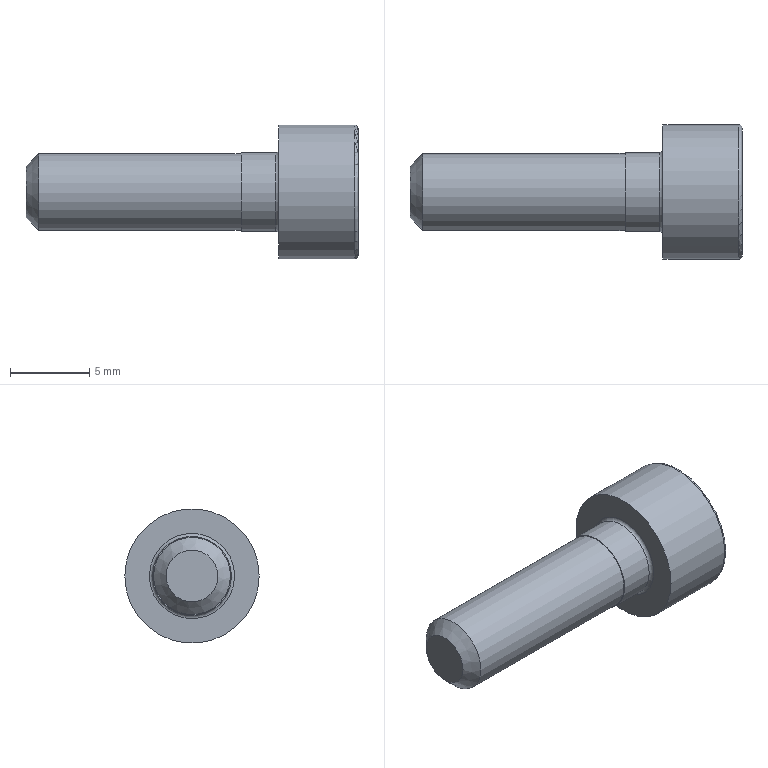Part | STEP file | DIN_912 - M5x16 | 1 solid | 24 faces | box 21 x 8.5 x 8.5 mm | volume 538.828 mm3 | plane 11 | cylinder 9 | torus 2 | cone 2 | commonest cylinder face diameters 4.583 x6 4.878 x1 5 x1 8.5 x1